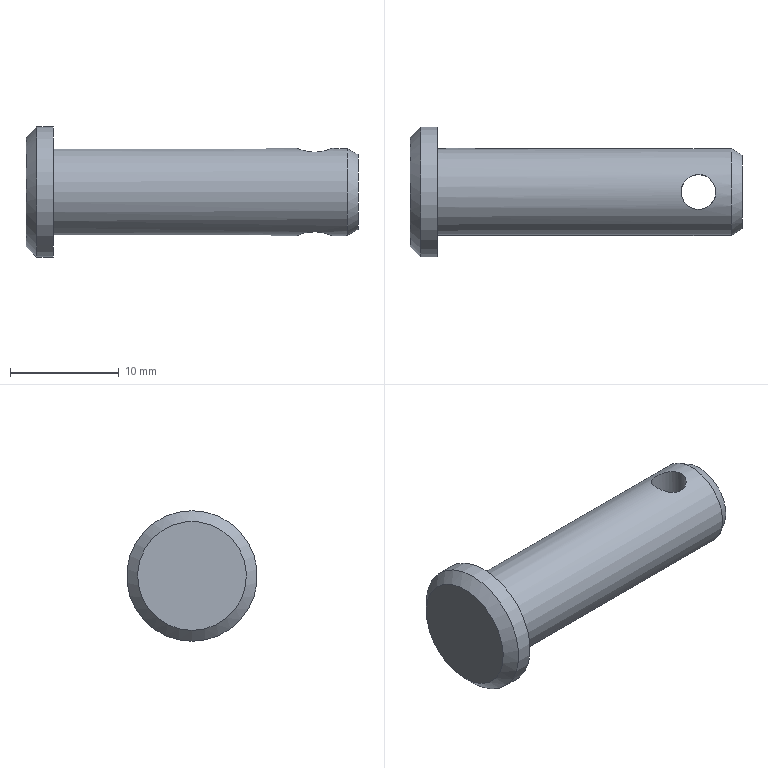Part | NX | features solid 2 | 1 solid | 8 faces | box 30.5 x 12 x 12 mm | volume 1602 mm3 | cylinder 3 | plane 3 | cone 2 | commonest cylinder face diameters 3.2 x1 8 x1 12 x1
STEP:
#1=CARTESIAN_POINT('',(280.6,-465.,-101.));
#2=VERTEX_POINT('',#1);
#3=CARTESIAN_POINT('',(280.253,-463.745,-100.84));
#4=CARTESIAN_POINT('',(280.774,-465.,-101.08));
#5=CARTESIAN_POINT('',(280.252,-466.254,-100.84));
#6=CARTESIAN_POINT('',(279.003,-466.773,-100.579));
#7=CARTESIAN_POINT('',(277.746,-466.254,-100.84));
#8=CARTESIAN_POINT('',(277.227,-465.003,-101.08));
#9=CARTESIAN_POINT('',(277.746,-463.746,-100.84));
#10=CARTESIAN_POINT('',(278.999,-463.227,-100.579));
#11=CARTESIAN_POINT('',(280.253,-463.745,-100.84));
#12=CARTESIAN_POINT('',(280.774,-465.,-101.08));
#13=CARTESIAN_POINT('',(280.252,-466.254,-100.84));
#14=B_SPLINE_CURVE_WITH_KNOTS('',3,(#3,#4,#5,#6,#7,#8,#9,#10,#11,#12,#13),.UNSPECIFIED.,.T.,.F.,(1,1,1,1,1,1,1,1,1,1,1,1,1,1,1),(-0.003791,-0.002527,-0.001264,0.,0.001264,0.002527,0.003791,0.005054,0.006318,0.007581,0.008845,0.01011,0.01137,0.01264,0.0139),.UNSPECIFIED.);
#15=EDGE_CURVE('',#2,#2,#14,.T.);
#16=ORIENTED_EDGE('',*,*,#15,.F.);
#17=EDGE_LOOP('',(#16));
#18=FACE_BOUND('',#17,.T.);
#19=CARTESIAN_POINT('',(282.,-465.,-101.));
#20=VERTEX_POINT('',#19);
#21=CARTESIAN_POINT('',(282.,-465.,-97.));
#22=DIRECTION('',(-1.,0.,0.));
#23=DIRECTION('',(0.,0.,-1.));
#24=AXIS2_PLACEMENT_3D('',#21,#22,#23);
#25=CIRCLE('',#24,4.);
#26=EDGE_CURVE('',#20,#20,#25,.T.);
#27=ORIENTED_EDGE('',*,*,#26,.T.);
#28=EDGE_LOOP('',(#27));
#29=FACE_BOUND('',#28,.T.);
#30=CARTESIAN_POINT('',(255.,-469.,-97.));
#31=VERTEX_POINT('',#30);
#32=CARTESIAN_POINT('',(255.,-465.,-97.));
#33=DIRECTION('',(-1.,0.,0.));
#34=DIRECTION('',(0.,-1.,0.));
#35=AXIS2_PLACEMENT_3D('',#32,#33,#34);
#36=CIRCLE('',#35,4.);
#37=EDGE_CURVE('',#31,#31,#36,.T.);
#38=ORIENTED_EDGE('',*,*,#37,.F.);
#39=EDGE_LOOP('',(#38));
#40=FACE_BOUND('',#39,.T.);
#41=CARTESIAN_POINT('',(277.4,-465.,-93.));
#42=VERTEX_POINT('',#41);
#43=CARTESIAN_POINT('',(277.747,-463.745,-93.16));
#44=CARTESIAN_POINT('',(277.226,-465.,-92.92));
#45=CARTESIAN_POINT('',(277.748,-466.254,-93.16));
#46=CARTESIAN_POINT('',(278.997,-466.773,-93.421));
#47=CARTESIAN_POINT('',(280.254,-466.254,-93.16));
#48=CARTESIAN_POINT('',(280.773,-465.003,-92.92));
#49=CARTESIAN_POINT('',(280.254,-463.746,-93.16));
#50=CARTESIAN_POINT('',(279.001,-463.227,-93.421));
#51=CARTESIAN_POINT('',(277.747,-463.745,-93.16));
#52=CARTESIAN_POINT('',(277.226,-465.,-92.92));
#53=CARTESIAN_POINT('',(277.748,-466.254,-93.16));
#54=B_SPLINE_CURVE_WITH_KNOTS('',3,(#43,#44,#45,#46,#47,#48,#49,#50,#51,#52,#53),.UNSPECIFIED.,.T.,.F.,(1,1,1,1,1,1,1,1,1,1,1,1,1,1,1),(-0.003791,-0.002527,-0.001264,0.,0.001264,0.002527,0.003791,0.005054,0.006318,0.007581,0.008845,0.01011,0.01137,0.01264,0.0139),.UNSPECIFIED.);
#55=EDGE_CURVE('',#42,#42,#54,.T.);
#56=ORIENTED_EDGE('',*,*,#55,.F.);
#57=EDGE_LOOP('',(#56));
#58=FACE_BOUND('',#57,.T.);
#59=CARTESIAN_POINT('',(252.5,-465.,-97.));
#60=DIRECTION('',(1.,0.,0.));
#61=DIRECTION('',(0.,0.,1.));
#62=AXIS2_PLACEMENT_3D('',#59,#60,#61);
#63=CYLINDRICAL_SURFACE('',#62,4.);
#64=ADVANCED_FACE('',(#18,#29,#40,#58),#63,.T.);
#65=CARTESIAN_POINT('',(283.,-465.,-100.423));
#66=VERTEX_POINT('',#65);
#67=CARTESIAN_POINT('',(283.,-465.,-97.));
#68=DIRECTION('',(-1.,0.,0.));
#69=DIRECTION('',(0.,0.,-1.));
#70=AXIS2_PLACEMENT_3D('',#67,#68,#69);
#71=CIRCLE('',#70,3.423);
#72=EDGE_CURVE('',#66,#66,#71,.F.);
#73=ORIENTED_EDGE('',*,*,#72,.T.);
#74=EDGE_LOOP('',(#73));
#75=FACE_BOUND('',#74,.T.);
#76=CARTESIAN_POINT('',(283.,-465.,-97.));
#77=DIRECTION('',(-1.,0.,0.));
#78=DIRECTION('',(0.,0.,-1.));
#79=AXIS2_PLACEMENT_3D('',#76,#77,#78);
#80=PLANE('',#79);
#81=ADVANCED_FACE('',(#75),#80,.F.);
#82=CARTESIAN_POINT('',(255.,-465.,-91.));
#83=VERTEX_POINT('',#82);
#84=CARTESIAN_POINT('',(255.,-465.,-97.));
#85=DIRECTION('',(1.,0.,0.));
#86=DIRECTION('',(0.,0.,1.));
#87=AXIS2_PLACEMENT_3D('',#84,#85,#86);
#88=CIRCLE('',#87,6.);
#89=EDGE_CURVE('',#83,#83,#88,.F.);
#90=ORIENTED_EDGE('',*,*,#89,.F.);
#91=EDGE_LOOP('',(#90));
#92=FACE_BOUND('',#91,.T.);
#93=ORIENTED_EDGE('',*,*,#37,.T.);
#94=EDGE_LOOP('',(#93));
#95=FACE_BOUND('',#94,.T.);
#96=CARTESIAN_POINT('',(255.,-465.,-97.));
#97=DIRECTION('',(1.,0.,0.));
#98=DIRECTION('',(0.,0.,1.));
#99=AXIS2_PLACEMENT_3D('',#96,#97,#98);
#100=PLANE('',#99);
#101=ADVANCED_FACE('',(#92,#95),#100,.T.);
#102=CARTESIAN_POINT('',(253.5,-465.,-103.));
#103=VERTEX_POINT('',#102);
#104=CARTESIAN_POINT('',(253.5,-465.,-97.));
#105=DIRECTION('',(-1.,0.,0.));
#106=DIRECTION('',(0.,0.,-1.));
#107=AXIS2_PLACEMENT_3D('',#104,#105,#106);
#108=CIRCLE('',#107,6.);
#109=EDGE_CURVE('',#103,#103,#108,.F.);
#110=ORIENTED_EDGE('',*,*,#109,.T.);
#111=EDGE_LOOP('',(#110));
#112=FACE_BOUND('',#111,.T.);
#113=ORIENTED_EDGE('',*,*,#89,.T.);
#114=EDGE_LOOP('',(#113));
#115=FACE_BOUND('',#114,.T.);
#116=CARTESIAN_POINT('',(252.5,-465.,-97.));
#117=DIRECTION('',(1.,0.,0.));
#118=DIRECTION('',(0.,0.,1.));
#119=AXIS2_PLACEMENT_3D('',#116,#117,#118);
#120=CYLINDRICAL_SURFACE('',#119,6.);
#121=ADVANCED_FACE('',(#112,#115),#120,.T.);
#122=CARTESIAN_POINT('',(252.5,-465.,-102.));
#123=VERTEX_POINT('',#122);
#124=CARTESIAN_POINT('',(252.5,-465.,-97.));
#125=DIRECTION('',(-1.,0.,0.));
#126=DIRECTION('',(0.,0.,-1.));
#127=AXIS2_PLACEMENT_3D('',#124,#125,#126);
#128=CIRCLE('',#127,5.);
#129=EDGE_CURVE('',#123,#123,#128,.T.);
#130=ORIENTED_EDGE('',*,*,#129,.T.);
#131=EDGE_LOOP('',(#130));
#132=FACE_BOUND('',#131,.T.);
#133=CARTESIAN_POINT('',(252.5,-465.,-97.));
#134=DIRECTION('',(-1.,0.,0.));
#135=DIRECTION('',(0.,0.,-1.));
#136=AXIS2_PLACEMENT_3D('',#133,#134,#135);
#137=PLANE('',#136);
#138=ADVANCED_FACE('',(#132),#137,.T.);
#139=ORIENTED_EDGE('',*,*,#109,.F.);
#140=EDGE_LOOP('',(#139));
#141=FACE_BOUND('',#140,.T.);
#142=ORIENTED_EDGE('',*,*,#129,.F.);
#143=EDGE_LOOP('',(#142));
#144=FACE_BOUND('',#143,.T.);
#145=CARTESIAN_POINT('',(252.5,-465.,-97.));
#146=DIRECTION('',(1.,0.,0.));
#147=DIRECTION('',(0.,0.,1.));
#148=AXIS2_PLACEMENT_3D('',#145,#146,#147);
#149=CONICAL_SURFACE('',#148,5.,0.7854);
#150=ADVANCED_FACE('',(#141,#144),#149,.T.);
#151=ORIENTED_EDGE('',*,*,#72,.F.);
#152=EDGE_LOOP('',(#151));
#153=FACE_BOUND('',#152,.T.);
#154=ORIENTED_EDGE('',*,*,#26,.F.);
#155=EDGE_LOOP('',(#154));
#156=FACE_BOUND('',#155,.T.);
#157=CARTESIAN_POINT('',(282.,-465.,-97.));
#158=DIRECTION('',(-1.,0.,0.));
#159=DIRECTION('',(0.,0.,-1.));
#160=AXIS2_PLACEMENT_3D('',#157,#158,#159);
#161=CONICAL_SURFACE('',#160,4.,0.5236);
#162=ADVANCED_FACE('',(#153,#156),#161,.T.);
#163=ORIENTED_EDGE('',*,*,#15,.T.);
#164=EDGE_LOOP('',(#163));
#165=FACE_BOUND('',#164,.T.);
#166=ORIENTED_EDGE('',*,*,#55,.T.);
#167=EDGE_LOOP('',(#166));
#168=FACE_BOUND('',#167,.T.);
#169=CARTESIAN_POINT('',(279.,-465.,-5.));
#170=DIRECTION('',(0.,0.,-1.));
#171=DIRECTION('',(1.,0.,0.));
#172=AXIS2_PLACEMENT_3D('',#169,#170,#171);
#173=CYLINDRICAL_SURFACE('',#172,1.6);
#174=ADVANCED_FACE('',(#165,#168),#173,.F.);
#175=CLOSED_SHELL('',(#64,#81,#101,#121,#138,#150,#162,#174));
#176=MANIFOLD_SOLID_BREP('',#175);
#177=(LENGTH_UNIT()NAMED_UNIT(*)SI_UNIT(.MILLI.,.METRE.));
#178=UNCERTAINTY_MEASURE_WITH_UNIT(LENGTH_MEASURE(0.0508),#177,'','');
#179=(NAMED_UNIT(*)PLANE_ANGLE_UNIT()SI_UNIT($,.RADIAN.));
#180=(NAMED_UNIT(*)SI_UNIT($,.STERADIAN.)SOLID_ANGLE_UNIT());
#181=(GEOMETRIC_REPRESENTATION_CONTEXT(3)GLOBAL_UNCERTAINTY_ASSIGNED_CONTEXT((#178))GLOBAL_UNIT_ASSIGNED_CONTEXT((#177,#179,#180))REPRESENTATION_CONTEXT('',''));
#182=ADVANCED_BREP_SHAPE_REPRESENTATION('',(#176),#181);